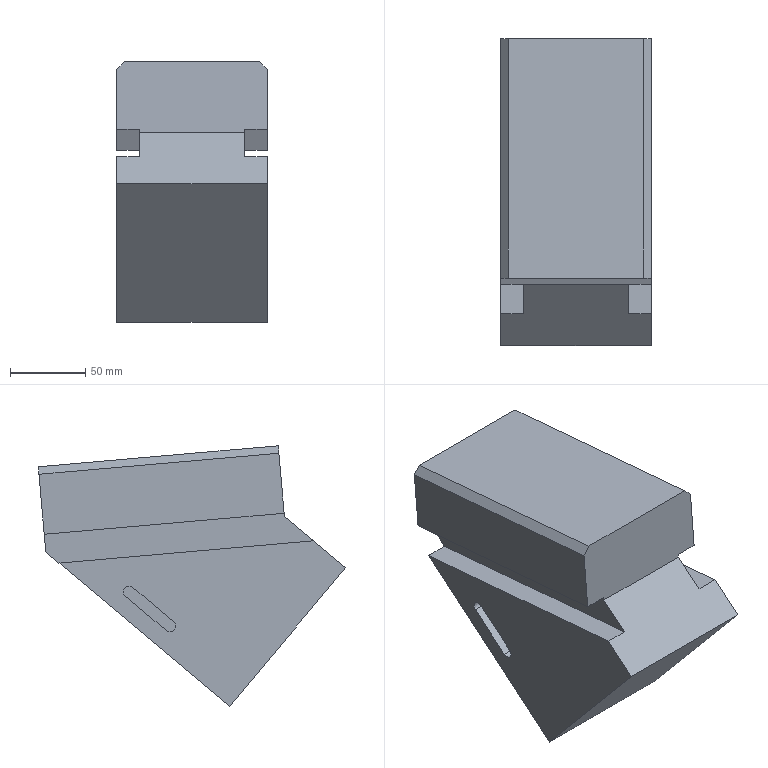Part | NX | features solid 2 | 1 solid | 28 faces | box 100 x 204.22 x 173.003 mm | volume 1996841 mm3 | plane 24 | cylinder 4 | commonest cylinder face diameters 7.661 x4
STEP:
#1=CARTESIAN_POINT('',(-480.,641.399,120.956));
#2=VERTEX_POINT('',#1);
#3=CARTESIAN_POINT('',(-480.,620.,103.));
#4=VERTEX_POINT('',#3);
#5=CARTESIAN_POINT('',(-480.,766.747,226.135));
#6=DIRECTION('',(0.,-0.766,-0.6428));
#7=VECTOR('',#6,1000.);
#8=LINE('',#5,#7);
#9=EDGE_CURVE('',#2,#4,#8,.T.);
#10=ORIENTED_EDGE('',*,*,#9,.T.);
#11=CARTESIAN_POINT('',(-480.,697.135,11.075));
#12=VERTEX_POINT('',#11);
#13=CARTESIAN_POINT('',(-480.,713.253,-8.135));
#14=DIRECTION('',(0.,0.6428,-0.766));
#15=VECTOR('',#14,1000.);
#16=LINE('',#13,#15);
#17=EDGE_CURVE('',#4,#12,#16,.T.);
#18=ORIENTED_EDGE('',*,*,#17,.T.);
#19=CARTESIAN_POINT('',(-480.,810.459,106.165));
#20=VERTEX_POINT('',#19);
#21=CARTESIAN_POINT('',(-480.,843.881,134.21));
#22=DIRECTION('',(0.,-0.766,-0.6428));
#23=VECTOR('',#22,1000.);
#24=LINE('',#21,#23);
#25=EDGE_CURVE('',#20,#12,#24,.T.);
#26=ORIENTED_EDGE('',*,*,#25,.F.);
#27=CARTESIAN_POINT('',(-480.,709.476,115.));
#28=DIRECTION('',(0.,-0.9962,0.08716));
#29=VECTOR('',#28,1000.);
#30=LINE('',#27,#29);
#31=EDGE_CURVE('',#20,#2,#30,.T.);
#32=ORIENTED_EDGE('',*,*,#31,.T.);
#33=EDGE_LOOP('',(#10,#18,#26,#32));
#34=FACE_BOUND('',#33,.T.);
#35=CARTESIAN_POINT('',(-480.,766.324,84.132));
#36=VERTEX_POINT('',#35);
#37=CARTESIAN_POINT('',(-480.,739.242,61.407));
#38=VERTEX_POINT('',#37);
#39=CARTESIAN_POINT('',(-480.,761.4,80.));
#40=DIRECTION('',(0.,-0.766,-0.6428));
#41=VECTOR('',#40,1000.);
#42=LINE('',#39,#41);
#43=EDGE_CURVE('',#36,#38,#42,.T.);
#44=ORIENTED_EDGE('',*,*,#43,.T.);
#45=CARTESIAN_POINT('',(-480.,734.318,67.275));
#46=VERTEX_POINT('',#45);
#47=CARTESIAN_POINT('',(-480.,736.765,64.329));
#48=DIRECTION('',(-1.,0.,0.));
#49=DIRECTION('',(0.,-1.,0.));
#50=AXIS2_PLACEMENT_3D('',#47,#48,#49);
#51=CIRCLE('',#50,3.83);
#52=EDGE_CURVE('',#38,#46,#51,.T.);
#53=ORIENTED_EDGE('',*,*,#52,.T.);
#54=CARTESIAN_POINT('',(-480.,761.4,90.));
#55=VERTEX_POINT('',#54);
#56=CARTESIAN_POINT('',(-480.,761.4,90.));
#57=DIRECTION('',(0.,-0.766,-0.6428));
#58=VECTOR('',#57,1000.);
#59=LINE('',#56,#58);
#60=EDGE_CURVE('',#55,#46,#59,.T.);
#61=ORIENTED_EDGE('',*,*,#60,.F.);
#62=CARTESIAN_POINT('',(-480.,763.874,87.076));
#63=DIRECTION('',(-1.,0.,0.));
#64=DIRECTION('',(0.,-1.,0.));
#65=AXIS2_PLACEMENT_3D('',#62,#63,#64);
#66=CIRCLE('',#65,3.83);
#67=EDGE_CURVE('',#55,#36,#66,.T.);
#68=ORIENTED_EDGE('',*,*,#67,.T.);
#69=EDGE_LOOP('',(#44,#53,#61,#68));
#70=FACE_BOUND('',#69,.T.);
#71=CARTESIAN_POINT('',(-480.,860.,115.));
#72=DIRECTION('',(1.,0.,0.));
#73=DIRECTION('',(0.,0.,-1.));
#74=AXIS2_PLACEMENT_3D('',#71,#72,#73);
#75=PLANE('',#74);
#76=ADVANCED_FACE('',(#34,#70),#75,.T.);
#77=CARTESIAN_POINT('',(-580.,761.4,90.));
#78=VERTEX_POINT('',#77);
#79=CARTESIAN_POINT('',(-580.,766.324,84.132));
#80=VERTEX_POINT('',#79);
#81=CARTESIAN_POINT('',(-580.,763.874,87.076));
#82=DIRECTION('',(-1.,0.,0.));
#83=DIRECTION('',(0.,-1.,0.));
#84=AXIS2_PLACEMENT_3D('',#81,#82,#83);
#85=CIRCLE('',#84,3.83);
#86=EDGE_CURVE('',#78,#80,#85,.T.);
#87=ORIENTED_EDGE('',*,*,#86,.F.);
#88=CARTESIAN_POINT('',(-580.,734.318,67.275));
#89=VERTEX_POINT('',#88);
#90=CARTESIAN_POINT('',(-580.,761.4,90.));
#91=DIRECTION('',(0.,-0.766,-0.6428));
#92=VECTOR('',#91,1000.);
#93=LINE('',#90,#92);
#94=EDGE_CURVE('',#78,#89,#93,.T.);
#95=ORIENTED_EDGE('',*,*,#94,.T.);
#96=CARTESIAN_POINT('',(-580.,739.242,61.407));
#97=VERTEX_POINT('',#96);
#98=CARTESIAN_POINT('',(-580.,736.765,64.329));
#99=DIRECTION('',(-1.,0.,0.));
#100=DIRECTION('',(0.,-1.,0.));
#101=AXIS2_PLACEMENT_3D('',#98,#99,#100);
#102=CIRCLE('',#101,3.83);
#103=EDGE_CURVE('',#97,#89,#102,.T.);
#104=ORIENTED_EDGE('',*,*,#103,.F.);
#105=CARTESIAN_POINT('',(-580.,761.4,80.));
#106=DIRECTION('',(0.,-0.766,-0.6428));
#107=VECTOR('',#106,1000.);
#108=LINE('',#105,#107);
#109=EDGE_CURVE('',#80,#97,#108,.T.);
#110=ORIENTED_EDGE('',*,*,#109,.F.);
#111=EDGE_LOOP('',(#87,#95,#104,#110));
#112=FACE_BOUND('',#111,.T.);
#113=CARTESIAN_POINT('',(-580.,810.459,106.165));
#114=VERTEX_POINT('',#113);
#115=CARTESIAN_POINT('',(-580.,641.399,120.956));
#116=VERTEX_POINT('',#115);
#117=CARTESIAN_POINT('',(-580.,709.476,115.));
#118=DIRECTION('',(0.,-0.9962,0.08716));
#119=VECTOR('',#118,1000.);
#120=LINE('',#117,#119);
#121=EDGE_CURVE('',#114,#116,#120,.T.);
#122=ORIENTED_EDGE('',*,*,#121,.F.);
#123=CARTESIAN_POINT('',(-580.,697.135,11.075));
#124=VERTEX_POINT('',#123);
#125=CARTESIAN_POINT('',(-580.,875.887,161.066));
#126=DIRECTION('',(0.,0.766,0.6428));
#127=VECTOR('',#126,1000.);
#128=LINE('',#125,#127);
#129=EDGE_CURVE('',#124,#114,#128,.T.);
#130=ORIENTED_EDGE('',*,*,#129,.F.);
#131=CARTESIAN_POINT('',(-580.,620.,103.));
#132=VERTEX_POINT('',#131);
#133=CARTESIAN_POINT('',(-580.,681.247,30.009));
#134=DIRECTION('',(0.,-0.6428,0.766));
#135=VECTOR('',#134,1000.);
#136=LINE('',#133,#135);
#137=EDGE_CURVE('',#124,#132,#136,.T.);
#138=ORIENTED_EDGE('',*,*,#137,.T.);
#139=CARTESIAN_POINT('',(-580.,798.753,252.991));
#140=DIRECTION('',(0.,0.766,0.6428));
#141=VECTOR('',#140,1000.);
#142=LINE('',#139,#141);
#143=EDGE_CURVE('',#132,#116,#142,.T.);
#144=ORIENTED_EDGE('',*,*,#143,.T.);
#145=EDGE_LOOP('',(#122,#130,#138,#144));
#146=FACE_BOUND('',#145,.T.);
#147=CARTESIAN_POINT('',(-580.,860.,180.));
#148=DIRECTION('',(-1.,0.,0.));
#149=DIRECTION('',(0.,1.,0.));
#150=AXIS2_PLACEMENT_3D('',#147,#148,#149);
#151=PLANE('',#150);
#152=ADVANCED_FACE('',(#112,#146),#151,.T.);
#153=CARTESIAN_POINT('',(-480.,823.784,165.152));
#154=VERTEX_POINT('',#153);
#155=CARTESIAN_POINT('',(-480.,820.298,125.304));
#156=VERTEX_POINT('',#155);
#157=CARTESIAN_POINT('',(-480.,819.705,118.525));
#158=DIRECTION('',(0.,-0.08716,-0.9962));
#159=VECTOR('',#158,1000.);
#160=LINE('',#157,#159);
#161=EDGE_CURVE('',#154,#156,#160,.T.);
#162=ORIENTED_EDGE('',*,*,#161,.F.);
#163=CARTESIAN_POINT('',(-480.,664.393,179.097));
#164=VERTEX_POINT('',#163);
#165=CARTESIAN_POINT('',(-480.,864.079,161.627));
#166=DIRECTION('',(0.,0.9962,-0.08716));
#167=VECTOR('',#166,1000.);
#168=LINE('',#165,#167);
#169=EDGE_CURVE('',#164,#154,#168,.T.);
#170=ORIENTED_EDGE('',*,*,#169,.F.);
#171=CARTESIAN_POINT('',(-480.,660.907,139.249));
#172=VERTEX_POINT('',#171);
#173=CARTESIAN_POINT('',(-480.,660.314,132.47));
#174=DIRECTION('',(0.,-0.08716,-0.9962));
#175=VECTOR('',#174,1000.);
#176=LINE('',#173,#175);
#177=EDGE_CURVE('',#164,#172,#176,.T.);
#178=ORIENTED_EDGE('',*,*,#177,.T.);
#179=CARTESIAN_POINT('',(-480.,820.,125.33));
#180=DIRECTION('',(0.,0.9962,-0.08716));
#181=VECTOR('',#180,1000.);
#182=LINE('',#179,#181);
#183=EDGE_CURVE('',#172,#156,#182,.T.);
#184=ORIENTED_EDGE('',*,*,#183,.T.);
#185=EDGE_LOOP('',(#162,#170,#178,#184));
#186=FACE_BOUND('',#185,.T.);
#187=CARTESIAN_POINT('',(-480.,860.,115.));
#188=DIRECTION('',(1.,0.,0.));
#189=DIRECTION('',(0.,0.,-1.));
#190=AXIS2_PLACEMENT_3D('',#187,#188,#189);
#191=PLANE('',#190);
#192=ADVANCED_FACE('',(#186),#191,.T.);
#193=CARTESIAN_POINT('',(-580.,820.298,125.304));
#194=VERTEX_POINT('',#193);
#195=CARTESIAN_POINT('',(-565.,820.298,125.304));
#196=VERTEX_POINT('',#195);
#197=CARTESIAN_POINT('',(-580.,820.298,125.304));
#198=DIRECTION('',(1.,0.,0.));
#199=VECTOR('',#198,1000.);
#200=LINE('',#197,#199);
#201=EDGE_CURVE('',#194,#196,#200,.T.);
#202=ORIENTED_EDGE('',*,*,#201,.F.);
#203=CARTESIAN_POINT('',(-580.,823.784,165.152));
#204=VERTEX_POINT('',#203);
#205=CARTESIAN_POINT('',(-580.,825.348,183.032));
#206=DIRECTION('',(0.,0.08716,0.9962));
#207=VECTOR('',#206,1000.);
#208=LINE('',#205,#207);
#209=EDGE_CURVE('',#194,#204,#208,.T.);
#210=ORIENTED_EDGE('',*,*,#209,.T.);
#211=CARTESIAN_POINT('',(-575.,824.22,170.133));
#212=VERTEX_POINT('',#211);
#213=CARTESIAN_POINT('',(-652.5,817.465,92.928));
#214=DIRECTION('',(0.7071,0.06163,0.7044));
#215=VECTOR('',#214,1000.);
#216=LINE('',#213,#215);
#217=EDGE_CURVE('',#212,#204,#216,.F.);
#218=ORIENTED_EDGE('',*,*,#217,.F.);
#219=CARTESIAN_POINT('',(-485.,824.22,170.133));
#220=VERTEX_POINT('',#219);
#221=CARTESIAN_POINT('',(-730.,824.22,170.133));
#222=DIRECTION('',(1.,0.,0.));
#223=VECTOR('',#222,1000.);
#224=LINE('',#221,#223);
#225=EDGE_CURVE('',#212,#220,#224,.T.);
#226=ORIENTED_EDGE('',*,*,#225,.T.);
#227=CARTESIAN_POINT('',(-607.5,834.896,292.167));
#228=DIRECTION('',(0.7071,-0.06163,-0.7044));
#229=VECTOR('',#228,1000.);
#230=LINE('',#227,#229);
#231=EDGE_CURVE('',#154,#220,#230,.F.);
#232=ORIENTED_EDGE('',*,*,#231,.F.);
#233=ORIENTED_EDGE('',*,*,#161,.T.);
#234=CARTESIAN_POINT('',(-495.,820.298,125.304));
#235=VERTEX_POINT('',#234);
#236=CARTESIAN_POINT('',(-480.,820.298,125.304));
#237=DIRECTION('',(-1.,0.,0.));
#238=VECTOR('',#237,1000.);
#239=LINE('',#236,#238);
#240=EDGE_CURVE('',#156,#235,#239,.T.);
#241=ORIENTED_EDGE('',*,*,#240,.T.);
#242=CARTESIAN_POINT('',(-495.,819.27,113.559));
#243=VERTEX_POINT('',#242);
#244=CARTESIAN_POINT('',(-495.,824.22,170.133));
#245=DIRECTION('',(0.,-0.08716,-0.9962));
#246=VECTOR('',#245,1000.);
#247=LINE('',#244,#246);
#248=EDGE_CURVE('',#235,#243,#247,.T.);
#249=ORIENTED_EDGE('',*,*,#248,.T.);
#250=CARTESIAN_POINT('',(-565.,819.27,113.559));
#251=VERTEX_POINT('',#250);
#252=CARTESIAN_POINT('',(-730.,819.27,113.559));
#253=DIRECTION('',(1.,0.,0.));
#254=VECTOR('',#253,1000.);
#255=LINE('',#252,#254);
#256=EDGE_CURVE('',#251,#243,#255,.T.);
#257=ORIENTED_EDGE('',*,*,#256,.F.);
#258=CARTESIAN_POINT('',(-565.,824.22,170.133));
#259=DIRECTION('',(0.,-0.08716,-0.9962));
#260=VECTOR('',#259,1000.);
#261=LINE('',#258,#260);
#262=EDGE_CURVE('',#196,#251,#261,.T.);
#263=ORIENTED_EDGE('',*,*,#262,.F.);
#264=EDGE_LOOP('',(#202,#210,#218,#226,#232,#233,#241,#249,#257,#263));
#265=FACE_BOUND('',#264,.T.);
#266=CARTESIAN_POINT('',(-730.,824.22,170.133));
#267=DIRECTION('',(0.,0.9962,-0.08716));
#268=DIRECTION('',(0.,-0.08716,-0.9962));
#269=AXIS2_PLACEMENT_3D('',#266,#267,#268);
#270=PLANE('',#269);
#271=ADVANCED_FACE('',(#265),#270,.T.);
#272=CARTESIAN_POINT('',(-565.,660.907,139.249));
#273=VERTEX_POINT('',#272);
#274=CARTESIAN_POINT('',(-565.,660.725,137.172));
#275=VERTEX_POINT('',#274);
#276=CARTESIAN_POINT('',(-565.,660.907,139.249));
#277=DIRECTION('',(0.,-0.08716,-0.9962));
#278=VECTOR('',#277,1000.);
#279=LINE('',#276,#278);
#280=EDGE_CURVE('',#273,#275,#279,.T.);
#281=ORIENTED_EDGE('',*,*,#280,.T.);
#282=CARTESIAN_POINT('',(-495.,660.725,137.172));
#283=VERTEX_POINT('',#282);
#284=CARTESIAN_POINT('',(-730.,660.725,137.172));
#285=DIRECTION('',(1.,0.,0.));
#286=VECTOR('',#285,1000.);
#287=LINE('',#284,#286);
#288=EDGE_CURVE('',#275,#283,#287,.T.);
#289=ORIENTED_EDGE('',*,*,#288,.T.);
#290=CARTESIAN_POINT('',(-495.,660.907,139.249));
#291=VERTEX_POINT('',#290);
#292=CARTESIAN_POINT('',(-495.,660.907,139.249));
#293=DIRECTION('',(0.,-0.08716,-0.9962));
#294=VECTOR('',#293,1000.);
#295=LINE('',#292,#294);
#296=EDGE_CURVE('',#291,#283,#295,.T.);
#297=ORIENTED_EDGE('',*,*,#296,.F.);
#298=CARTESIAN_POINT('',(-480.,660.907,139.249));
#299=DIRECTION('',(-1.,0.,0.));
#300=VECTOR('',#299,1000.);
#301=LINE('',#298,#300);
#302=EDGE_CURVE('',#172,#291,#301,.T.);
#303=ORIENTED_EDGE('',*,*,#302,.F.);
#304=ORIENTED_EDGE('',*,*,#177,.F.);
#305=CARTESIAN_POINT('',(-485.,664.829,184.078));
#306=VERTEX_POINT('',#305);
#307=CARTESIAN_POINT('',(-480.,664.393,179.097));
#308=DIRECTION('',(-0.7071,0.06163,0.7044));
#309=VECTOR('',#308,1000.);
#310=LINE('',#307,#309);
#311=EDGE_CURVE('',#306,#164,#310,.F.);
#312=ORIENTED_EDGE('',*,*,#311,.F.);
#313=CARTESIAN_POINT('',(-575.,664.829,184.078));
#314=VERTEX_POINT('',#313);
#315=CARTESIAN_POINT('',(-730.,664.829,184.078));
#316=DIRECTION('',(1.,0.,0.));
#317=VECTOR('',#316,1000.);
#318=LINE('',#315,#317);
#319=EDGE_CURVE('',#314,#306,#318,.T.);
#320=ORIENTED_EDGE('',*,*,#319,.F.);
#321=CARTESIAN_POINT('',(-580.,664.393,179.097));
#322=VERTEX_POINT('',#321);
#323=CARTESIAN_POINT('',(-580.,664.393,179.097));
#324=DIRECTION('',(-0.7071,-0.06163,-0.7044));
#325=VECTOR('',#324,1000.);
#326=LINE('',#323,#325);
#327=EDGE_CURVE('',#322,#314,#326,.F.);
#328=ORIENTED_EDGE('',*,*,#327,.F.);
#329=CARTESIAN_POINT('',(-580.,660.907,139.249));
#330=VERTEX_POINT('',#329);
#331=CARTESIAN_POINT('',(-580.,665.957,196.977));
#332=DIRECTION('',(0.,0.08716,0.9962));
#333=VECTOR('',#332,1000.);
#334=LINE('',#331,#333);
#335=EDGE_CURVE('',#330,#322,#334,.T.);
#336=ORIENTED_EDGE('',*,*,#335,.F.);
#337=CARTESIAN_POINT('',(-580.,660.907,139.249));
#338=DIRECTION('',(1.,0.,0.));
#339=VECTOR('',#338,1000.);
#340=LINE('',#337,#339);
#341=EDGE_CURVE('',#330,#273,#340,.T.);
#342=ORIENTED_EDGE('',*,*,#341,.T.);
#343=EDGE_LOOP('',(#281,#289,#297,#303,#304,#312,#320,#328,#336,#342));
#344=FACE_BOUND('',#343,.T.);
#345=CARTESIAN_POINT('',(-730.,660.907,139.249));
#346=DIRECTION('',(0.,0.9962,-0.08716));
#347=DIRECTION('',(0.,-0.08716,-0.9962));
#348=AXIS2_PLACEMENT_3D('',#345,#346,#347);
#349=PLANE('',#348);
#350=ADVANCED_FACE('',(#344),#349,.F.);
#351=ORIENTED_EDGE('',*,*,#143,.F.);
#352=CARTESIAN_POINT('',(-730.,620.,103.));
#353=DIRECTION('',(1.,0.,0.));
#354=VECTOR('',#353,1000.);
#355=LINE('',#352,#354);
#356=EDGE_CURVE('',#132,#4,#355,.T.);
#357=ORIENTED_EDGE('',*,*,#356,.T.);
#358=ORIENTED_EDGE('',*,*,#9,.F.);
#359=CARTESIAN_POINT('',(-495.,641.399,120.956));
#360=VERTEX_POINT('',#359);
#361=CARTESIAN_POINT('',(-730.,641.399,120.956));
#362=DIRECTION('',(-1.,0.,0.));
#363=VECTOR('',#362,1000.);
#364=LINE('',#361,#363);
#365=EDGE_CURVE('',#2,#360,#364,.T.);
#366=ORIENTED_EDGE('',*,*,#365,.T.);
#367=CARTESIAN_POINT('',(-495.,660.725,137.172));
#368=DIRECTION('',(0.,-0.766,-0.6428));
#369=VECTOR('',#368,1000.);
#370=LINE('',#367,#369);
#371=EDGE_CURVE('',#283,#360,#370,.T.);
#372=ORIENTED_EDGE('',*,*,#371,.F.);
#373=ORIENTED_EDGE('',*,*,#288,.F.);
#374=CARTESIAN_POINT('',(-565.,641.399,120.956));
#375=VERTEX_POINT('',#374);
#376=CARTESIAN_POINT('',(-565.,660.725,137.172));
#377=DIRECTION('',(0.,-0.766,-0.6428));
#378=VECTOR('',#377,1000.);
#379=LINE('',#376,#378);
#380=EDGE_CURVE('',#275,#375,#379,.T.);
#381=ORIENTED_EDGE('',*,*,#380,.T.);
#382=CARTESIAN_POINT('',(-730.,641.399,120.956));
#383=DIRECTION('',(1.,0.,0.));
#384=VECTOR('',#383,1000.);
#385=LINE('',#382,#384);
#386=EDGE_CURVE('',#116,#375,#385,.T.);
#387=ORIENTED_EDGE('',*,*,#386,.F.);
#388=EDGE_LOOP('',(#351,#357,#358,#366,#372,#373,#381,#387));
#389=FACE_BOUND('',#388,.T.);
#390=CARTESIAN_POINT('',(-730.,660.725,137.172));
#391=DIRECTION('',(0.,0.6428,-0.766));
#392=DIRECTION('',(0.,-0.766,-0.6428));
#393=AXIS2_PLACEMENT_3D('',#390,#391,#392);
#394=PLANE('',#393);
#395=ADVANCED_FACE('',(#389),#394,.F.);
#396=CARTESIAN_POINT('',(-565.,810.459,106.165));
#397=VERTEX_POINT('',#396);
#398=CARTESIAN_POINT('',(-580.,810.459,106.165));
#399=DIRECTION('',(1.,0.,0.));
#400=VECTOR('',#399,1000.);
#401=LINE('',#398,#400);
#402=EDGE_CURVE('',#114,#397,#401,.T.);
#403=ORIENTED_EDGE('',*,*,#402,.T.);
#404=CARTESIAN_POINT('',(-565.,819.27,113.559));
#405=DIRECTION('',(0.,-0.766,-0.6428));
#406=VECTOR('',#405,1000.);
#407=LINE('',#404,#406);
#408=EDGE_CURVE('',#251,#397,#407,.T.);
#409=ORIENTED_EDGE('',*,*,#408,.F.);
#410=ORIENTED_EDGE('',*,*,#256,.T.);
#411=CARTESIAN_POINT('',(-495.,810.459,106.165));
#412=VERTEX_POINT('',#411);
#413=CARTESIAN_POINT('',(-495.,819.27,113.559));
#414=DIRECTION('',(0.,-0.766,-0.6428));
#415=VECTOR('',#414,1000.);
#416=LINE('',#413,#415);
#417=EDGE_CURVE('',#243,#412,#416,.T.);
#418=ORIENTED_EDGE('',*,*,#417,.T.);
#419=CARTESIAN_POINT('',(-480.,810.459,106.165));
#420=DIRECTION('',(-1.,0.,0.));
#421=VECTOR('',#420,1000.);
#422=LINE('',#419,#421);
#423=EDGE_CURVE('',#20,#412,#422,.T.);
#424=ORIENTED_EDGE('',*,*,#423,.F.);
#425=ORIENTED_EDGE('',*,*,#25,.T.);
#426=CARTESIAN_POINT('',(-730.,697.135,11.075));
#427=DIRECTION('',(1.,0.,0.));
#428=VECTOR('',#427,1000.);
#429=LINE('',#426,#428);
#430=EDGE_CURVE('',#124,#12,#429,.T.);
#431=ORIENTED_EDGE('',*,*,#430,.F.);
#432=ORIENTED_EDGE('',*,*,#129,.T.);
#433=EDGE_LOOP('',(#403,#409,#410,#418,#424,#425,#431,#432));
#434=FACE_BOUND('',#433,.T.);
#435=CARTESIAN_POINT('',(-730.,819.27,113.559));
#436=DIRECTION('',(0.,0.6428,-0.766));
#437=DIRECTION('',(0.,-0.766,-0.6428));
#438=AXIS2_PLACEMENT_3D('',#435,#436,#437);
#439=PLANE('',#438);
#440=ADVANCED_FACE('',(#434),#439,.T.);
#441=ORIENTED_EDGE('',*,*,#319,.T.);
#442=CARTESIAN_POINT('',(-485.,654.867,184.95));
#443=DIRECTION('',(0.,-0.9962,0.08716));
#444=VECTOR('',#443,1000.);
#445=LINE('',#442,#444);
#446=EDGE_CURVE('',#220,#306,#445,.T.);
#447=ORIENTED_EDGE('',*,*,#446,.F.);
#448=ORIENTED_EDGE('',*,*,#225,.F.);
#449=CARTESIAN_POINT('',(-575.,654.867,184.95));
#450=DIRECTION('',(0.,0.9962,-0.08716));
#451=VECTOR('',#450,1000.);
#452=LINE('',#449,#451);
#453=EDGE_CURVE('',#314,#212,#452,.T.);
#454=ORIENTED_EDGE('',*,*,#453,.F.);
#455=EDGE_LOOP('',(#441,#447,#448,#454));
#456=FACE_BOUND('',#455,.T.);
#457=CARTESIAN_POINT('',(-730.,654.867,184.95));
#458=DIRECTION('',(0.,0.08716,0.9962));
#459=DIRECTION('',(0.,0.9962,-0.08716));
#460=AXIS2_PLACEMENT_3D('',#457,#458,#459);
#461=PLANE('',#460);
#462=ADVANCED_FACE('',(#456),#461,.T.);
#463=ORIENTED_EDGE('',*,*,#430,.T.);
#464=ORIENTED_EDGE('',*,*,#17,.F.);
#465=ORIENTED_EDGE('',*,*,#356,.F.);
#466=ORIENTED_EDGE('',*,*,#137,.F.);
#467=EDGE_LOOP('',(#463,#464,#465,#466));
#468=FACE_BOUND('',#467,.T.);
#469=CARTESIAN_POINT('',(-730.,620.,103.));
#470=DIRECTION('',(0.,0.766,0.6428));
#471=DIRECTION('',(0.,0.6428,-0.766));
#472=AXIS2_PLACEMENT_3D('',#469,#470,#471);
#473=PLANE('',#472);
#474=ADVANCED_FACE('',(#468),#473,.F.);
#475=CARTESIAN_POINT('',(-580.,820.,125.33));
#476=DIRECTION('',(0.,0.9962,-0.08716));
#477=VECTOR('',#476,1000.);
#478=LINE('',#475,#477);
#479=EDGE_CURVE('',#330,#194,#478,.T.);
#480=ORIENTED_EDGE('',*,*,#479,.F.);
#481=ORIENTED_EDGE('',*,*,#335,.T.);
#482=CARTESIAN_POINT('',(-580.,858.436,162.12));
#483=DIRECTION('',(0.,-0.9962,0.08716));
#484=VECTOR('',#483,1000.);
#485=LINE('',#482,#484);
#486=EDGE_CURVE('',#204,#322,#485,.T.);
#487=ORIENTED_EDGE('',*,*,#486,.F.);
#488=ORIENTED_EDGE('',*,*,#209,.F.);
#489=EDGE_LOOP('',(#480,#481,#487,#488));
#490=FACE_BOUND('',#489,.T.);
#491=CARTESIAN_POINT('',(-580.,860.,180.));
#492=DIRECTION('',(-1.,0.,0.));
#493=DIRECTION('',(0.,1.,0.));
#494=AXIS2_PLACEMENT_3D('',#491,#492,#493);
#495=PLANE('',#494);
#496=ADVANCED_FACE('',(#490),#495,.T.);
#497=ORIENTED_EDGE('',*,*,#217,.T.);
#498=ORIENTED_EDGE('',*,*,#486,.T.);
#499=ORIENTED_EDGE('',*,*,#327,.T.);
#500=ORIENTED_EDGE('',*,*,#453,.T.);
#501=EDGE_LOOP('',(#497,#498,#499,#500));
#502=FACE_BOUND('',#501,.T.);
#503=CARTESIAN_POINT('',(-580.,858.436,162.12));
#504=DIRECTION('',(0.7071,-0.06163,-0.7044));
#505=DIRECTION('',(-0.7058,0.,-0.7085));
#506=AXIS2_PLACEMENT_3D('',#503,#504,#505);
#507=PLANE('',#506);
#508=ADVANCED_FACE('',(#502),#507,.F.);
#509=ORIENTED_EDGE('',*,*,#311,.T.);
#510=ORIENTED_EDGE('',*,*,#169,.T.);
#511=ORIENTED_EDGE('',*,*,#231,.T.);
#512=ORIENTED_EDGE('',*,*,#446,.T.);
#513=EDGE_LOOP('',(#509,#510,#511,#512));
#514=FACE_BOUND('',#513,.T.);
#515=CARTESIAN_POINT('',(-480.,864.079,161.627));
#516=DIRECTION('',(-0.7071,-0.06163,-0.7044));
#517=DIRECTION('',(-0.7058,0.,0.7085));
#518=AXIS2_PLACEMENT_3D('',#515,#516,#517);
#519=PLANE('',#518);
#520=ADVANCED_FACE('',(#514),#519,.F.);
#521=CARTESIAN_POINT('',(-495.,709.476,115.));
#522=DIRECTION('',(0.,-0.9962,0.08716));
#523=VECTOR('',#522,1000.);
#524=LINE('',#521,#523);
#525=EDGE_CURVE('',#412,#360,#524,.T.);
#526=ORIENTED_EDGE('',*,*,#525,.T.);
#527=ORIENTED_EDGE('',*,*,#365,.F.);
#528=ORIENTED_EDGE('',*,*,#31,.F.);
#529=ORIENTED_EDGE('',*,*,#423,.T.);
#530=EDGE_LOOP('',(#526,#527,#528,#529));
#531=FACE_BOUND('',#530,.T.);
#532=CARTESIAN_POINT('',(-480.,709.476,115.));
#533=DIRECTION('',(0.,0.08716,0.9962));
#534=DIRECTION('',(0.,0.9962,-0.08716));
#535=AXIS2_PLACEMENT_3D('',#532,#533,#534);
#536=PLANE('',#535);
#537=ADVANCED_FACE('',(#531),#536,.T.);
#538=CARTESIAN_POINT('',(-495.,820.,125.33));
#539=DIRECTION('',(0.,0.9962,-0.08716));
#540=VECTOR('',#539,1000.);
#541=LINE('',#538,#540);
#542=EDGE_CURVE('',#291,#235,#541,.T.);
#543=ORIENTED_EDGE('',*,*,#542,.T.);
#544=ORIENTED_EDGE('',*,*,#240,.F.);
#545=ORIENTED_EDGE('',*,*,#183,.F.);
#546=ORIENTED_EDGE('',*,*,#302,.T.);
#547=EDGE_LOOP('',(#543,#544,#545,#546));
#548=FACE_BOUND('',#547,.T.);
#549=CARTESIAN_POINT('',(-480.,820.,125.33));
#550=DIRECTION('',(0.,-0.08716,-0.9962));
#551=DIRECTION('',(0.,-0.9962,0.08716));
#552=AXIS2_PLACEMENT_3D('',#549,#550,#551);
#553=PLANE('',#552);
#554=ADVANCED_FACE('',(#548),#553,.T.);
#555=ORIENTED_EDGE('',*,*,#525,.F.);
#556=ORIENTED_EDGE('',*,*,#417,.F.);
#557=ORIENTED_EDGE('',*,*,#248,.F.);
#558=ORIENTED_EDGE('',*,*,#542,.F.);
#559=ORIENTED_EDGE('',*,*,#296,.T.);
#560=ORIENTED_EDGE('',*,*,#371,.T.);
#561=EDGE_LOOP('',(#555,#556,#557,#558,#559,#560));
#562=FACE_BOUND('',#561,.T.);
#563=CARTESIAN_POINT('',(-495.,734.642,118.578));
#564=DIRECTION('',(-1.,0.,0.));
#565=DIRECTION('',(0.,1.,0.));
#566=AXIS2_PLACEMENT_3D('',#563,#564,#565);
#567=PLANE('',#566);
#568=ADVANCED_FACE('',(#562),#567,.F.);
#569=CARTESIAN_POINT('',(-565.,709.476,115.));
#570=DIRECTION('',(0.,-0.9962,0.08716));
#571=VECTOR('',#570,1000.);
#572=LINE('',#569,#571);
#573=EDGE_CURVE('',#397,#375,#572,.T.);
#574=ORIENTED_EDGE('',*,*,#573,.F.);
#575=ORIENTED_EDGE('',*,*,#402,.F.);
#576=ORIENTED_EDGE('',*,*,#121,.T.);
#577=ORIENTED_EDGE('',*,*,#386,.T.);
#578=EDGE_LOOP('',(#574,#575,#576,#577));
#579=FACE_BOUND('',#578,.T.);
#580=CARTESIAN_POINT('',(-580.,709.476,115.));
#581=DIRECTION('',(0.,-0.08716,-0.9962));
#582=DIRECTION('',(0.,-0.9962,0.08716));
#583=AXIS2_PLACEMENT_3D('',#580,#581,#582);
#584=PLANE('',#583);
#585=ADVANCED_FACE('',(#579),#584,.F.);
#586=CARTESIAN_POINT('',(-565.,820.,125.33));
#587=DIRECTION('',(0.,0.9962,-0.08716));
#588=VECTOR('',#587,1000.);
#589=LINE('',#586,#588);
#590=EDGE_CURVE('',#273,#196,#589,.T.);
#591=ORIENTED_EDGE('',*,*,#590,.F.);
#592=ORIENTED_EDGE('',*,*,#341,.F.);
#593=ORIENTED_EDGE('',*,*,#479,.T.);
#594=ORIENTED_EDGE('',*,*,#201,.T.);
#595=EDGE_LOOP('',(#591,#592,#593,#594));
#596=FACE_BOUND('',#595,.T.);
#597=CARTESIAN_POINT('',(-580.,820.,125.33));
#598=DIRECTION('',(0.,0.08716,0.9962));
#599=DIRECTION('',(0.,0.9962,-0.08716));
#600=AXIS2_PLACEMENT_3D('',#597,#598,#599);
#601=PLANE('',#600);
#602=ADVANCED_FACE('',(#596),#601,.F.);
#603=ORIENTED_EDGE('',*,*,#573,.T.);
#604=ORIENTED_EDGE('',*,*,#380,.F.);
#605=ORIENTED_EDGE('',*,*,#280,.F.);
#606=ORIENTED_EDGE('',*,*,#590,.T.);
#607=ORIENTED_EDGE('',*,*,#262,.T.);
#608=ORIENTED_EDGE('',*,*,#408,.T.);
#609=EDGE_LOOP('',(#603,#604,#605,#606,#607,#608));
#610=FACE_BOUND('',#609,.T.);
#611=CARTESIAN_POINT('',(-565.,734.642,118.578));
#612=DIRECTION('',(-1.,0.,0.));
#613=DIRECTION('',(0.,1.,0.));
#614=AXIS2_PLACEMENT_3D('',#611,#612,#613);
#615=PLANE('',#614);
#616=ADVANCED_FACE('',(#610),#615,.T.);
#617=CARTESIAN_POINT('',(-570.,761.4,90.));
#618=VERTEX_POINT('',#617);
#619=CARTESIAN_POINT('',(-570.,766.324,84.132));
#620=VERTEX_POINT('',#619);
#621=CARTESIAN_POINT('',(-570.,763.874,87.076));
#622=DIRECTION('',(-1.,0.,0.));
#623=DIRECTION('',(0.,-1.,0.));
#624=AXIS2_PLACEMENT_3D('',#621,#622,#623);
#625=CIRCLE('',#624,3.83);
#626=EDGE_CURVE('',#618,#620,#625,.T.);
#627=ORIENTED_EDGE('',*,*,#626,.F.);
#628=CARTESIAN_POINT('',(-580.,761.4,90.));
#629=DIRECTION('',(1.,0.,0.));
#630=VECTOR('',#629,1000.);
#631=LINE('',#628,#630);
#632=EDGE_CURVE('',#78,#618,#631,.T.);
#633=ORIENTED_EDGE('',*,*,#632,.F.);
#634=ORIENTED_EDGE('',*,*,#86,.T.);
#635=CARTESIAN_POINT('',(-580.,766.324,84.132));
#636=DIRECTION('',(1.,0.,0.));
#637=VECTOR('',#636,1000.);
#638=LINE('',#635,#637);
#639=EDGE_CURVE('',#80,#620,#638,.T.);
#640=ORIENTED_EDGE('',*,*,#639,.T.);
#641=EDGE_LOOP('',(#627,#633,#634,#640));
#642=FACE_BOUND('',#641,.T.);
#643=CARTESIAN_POINT('',(-580.,763.874,87.076));
#644=DIRECTION('',(1.,0.,0.));
#645=DIRECTION('',(0.,-1.,0.));
#646=AXIS2_PLACEMENT_3D('',#643,#644,#645);
#647=CYLINDRICAL_SURFACE('',#646,3.83);
#648=ADVANCED_FACE('',(#642),#647,.F.);
#649=CARTESIAN_POINT('',(-570.,739.242,61.407));
#650=VERTEX_POINT('',#649);
#651=CARTESIAN_POINT('',(-570.,761.4,80.));
#652=DIRECTION('',(0.,-0.766,-0.6428));
#653=VECTOR('',#652,1000.);
#654=LINE('',#651,#653);
#655=EDGE_CURVE('',#620,#650,#654,.T.);
#656=ORIENTED_EDGE('',*,*,#655,.F.);
#657=ORIENTED_EDGE('',*,*,#639,.F.);
#658=ORIENTED_EDGE('',*,*,#109,.T.);
#659=CARTESIAN_POINT('',(-580.,739.242,61.407));
#660=DIRECTION('',(1.,0.,0.));
#661=VECTOR('',#660,1000.);
#662=LINE('',#659,#661);
#663=EDGE_CURVE('',#97,#650,#662,.T.);
#664=ORIENTED_EDGE('',*,*,#663,.T.);
#665=EDGE_LOOP('',(#656,#657,#658,#664));
#666=FACE_BOUND('',#665,.T.);
#667=CARTESIAN_POINT('',(-580.,761.4,80.));
#668=DIRECTION('',(0.,0.6428,-0.766));
#669=DIRECTION('',(0.,-0.766,-0.6428));
#670=AXIS2_PLACEMENT_3D('',#667,#668,#669);
#671=PLANE('',#670);
#672=ADVANCED_FACE('',(#666),#671,.F.);
#673=CARTESIAN_POINT('',(-570.,734.318,67.275));
#674=VERTEX_POINT('',#673);
#675=CARTESIAN_POINT('',(-570.,736.765,64.329));
#676=DIRECTION('',(-1.,0.,0.));
#677=DIRECTION('',(0.,-1.,0.));
#678=AXIS2_PLACEMENT_3D('',#675,#676,#677);
#679=CIRCLE('',#678,3.83);
#680=EDGE_CURVE('',#650,#674,#679,.T.);
#681=ORIENTED_EDGE('',*,*,#680,.F.);
#682=ORIENTED_EDGE('',*,*,#663,.F.);
#683=ORIENTED_EDGE('',*,*,#103,.T.);
#684=CARTESIAN_POINT('',(-580.,734.318,67.275));
#685=DIRECTION('',(1.,0.,0.));
#686=VECTOR('',#685,1000.);
#687=LINE('',#684,#686);
#688=EDGE_CURVE('',#89,#674,#687,.T.);
#689=ORIENTED_EDGE('',*,*,#688,.T.);
#690=EDGE_LOOP('',(#681,#682,#683,#689));
#691=FACE_BOUND('',#690,.T.);
#692=CARTESIAN_POINT('',(-580.,736.765,64.329));
#693=DIRECTION('',(1.,0.,0.));
#694=DIRECTION('',(0.,-1.,0.));
#695=AXIS2_PLACEMENT_3D('',#692,#693,#694);
#696=CYLINDRICAL_SURFACE('',#695,3.83);
#697=ADVANCED_FACE('',(#691),#696,.F.);
#698=CARTESIAN_POINT('',(-570.,761.4,90.));
#699=DIRECTION('',(0.,-0.766,-0.6428));
#700=VECTOR('',#699,1000.);
#701=LINE('',#698,#700);
#702=EDGE_CURVE('',#618,#674,#701,.T.);
#703=ORIENTED_EDGE('',*,*,#702,.T.);
#704=ORIENTED_EDGE('',*,*,#688,.F.);
#705=ORIENTED_EDGE('',*,*,#94,.F.);
#706=ORIENTED_EDGE('',*,*,#632,.T.);
#707=EDGE_LOOP('',(#703,#704,#705,#706));
#708=FACE_BOUND('',#707,.T.);
#709=CARTESIAN_POINT('',(-580.,761.4,90.));
#710=DIRECTION('',(0.,0.6428,-0.766));
#711=DIRECTION('',(0.,-0.766,-0.6428));
#712=AXIS2_PLACEMENT_3D('',#709,#710,#711);
#713=PLANE('',#712);
#714=ADVANCED_FACE('',(#708),#713,.T.);
#715=ORIENTED_EDGE('',*,*,#626,.T.);
#716=ORIENTED_EDGE('',*,*,#655,.T.);
#717=ORIENTED_EDGE('',*,*,#680,.T.);
#718=ORIENTED_EDGE('',*,*,#702,.F.);
#719=EDGE_LOOP('',(#715,#716,#717,#718));
#720=FACE_BOUND('',#719,.T.);
#721=CARTESIAN_POINT('',(-570.,763.874,87.076));
#722=DIRECTION('',(1.,0.,0.));
#723=DIRECTION('',(0.,-1.,0.));
#724=AXIS2_PLACEMENT_3D('',#721,#722,#723);
#725=PLANE('',#724);
#726=ADVANCED_FACE('',(#720),#725,.F.);
#727=CARTESIAN_POINT('',(-490.,761.4,90.));
#728=VERTEX_POINT('',#727);
#729=CARTESIAN_POINT('',(-490.,766.324,84.132));
#730=VERTEX_POINT('',#729);
#731=CARTESIAN_POINT('',(-490.,763.874,87.076));
#732=DIRECTION('',(-1.,0.,0.));
#733=DIRECTION('',(0.,-1.,0.));
#734=AXIS2_PLACEMENT_3D('',#731,#732,#733);
#735=CIRCLE('',#734,3.83);
#736=EDGE_CURVE('',#728,#730,#735,.T.);
#737=ORIENTED_EDGE('',*,*,#736,.T.);
#738=CARTESIAN_POINT('',(-480.,766.324,84.132));
#739=DIRECTION('',(-1.,0.,0.));
#740=VECTOR('',#739,1000.);
#741=LINE('',#738,#740);
#742=EDGE_CURVE('',#36,#730,#741,.T.);
#743=ORIENTED_EDGE('',*,*,#742,.F.);
#744=ORIENTED_EDGE('',*,*,#67,.F.);
#745=CARTESIAN_POINT('',(-480.,761.4,90.));
#746=DIRECTION('',(-1.,0.,0.));
#747=VECTOR('',#746,1000.);
#748=LINE('',#745,#747);
#749=EDGE_CURVE('',#55,#728,#748,.T.);
#750=ORIENTED_EDGE('',*,*,#749,.T.);
#751=EDGE_LOOP('',(#737,#743,#744,#750));
#752=FACE_BOUND('',#751,.T.);
#753=CARTESIAN_POINT('',(-480.,763.874,87.076));
#754=DIRECTION('',(-1.,0.,0.));
#755=DIRECTION('',(0.,1.,0.));
#756=AXIS2_PLACEMENT_3D('',#753,#754,#755);
#757=CYLINDRICAL_SURFACE('',#756,3.83);
#758=ADVANCED_FACE('',(#752),#757,.F.);
#759=CARTESIAN_POINT('',(-490.,734.318,67.275));
#760=VERTEX_POINT('',#759);
#761=CARTESIAN_POINT('',(-490.,761.4,90.));
#762=DIRECTION('',(0.,-0.766,-0.6428));
#763=VECTOR('',#762,1000.);
#764=LINE('',#761,#763);
#765=EDGE_CURVE('',#728,#760,#764,.T.);
#766=ORIENTED_EDGE('',*,*,#765,.F.);
#767=ORIENTED_EDGE('',*,*,#749,.F.);
#768=ORIENTED_EDGE('',*,*,#60,.T.);
#769=CARTESIAN_POINT('',(-480.,734.318,67.275));
#770=DIRECTION('',(-1.,0.,0.));
#771=VECTOR('',#770,1000.);
#772=LINE('',#769,#771);
#773=EDGE_CURVE('',#46,#760,#772,.T.);
#774=ORIENTED_EDGE('',*,*,#773,.T.);
#775=EDGE_LOOP('',(#766,#767,#768,#774));
#776=FACE_BOUND('',#775,.T.);
#777=CARTESIAN_POINT('',(-480.,761.4,90.));
#778=DIRECTION('',(0.,-0.6428,0.766));
#779=DIRECTION('',(0.,0.766,0.6428));
#780=AXIS2_PLACEMENT_3D('',#777,#778,#779);
#781=PLANE('',#780);
#782=ADVANCED_FACE('',(#776),#781,.F.);
#783=CARTESIAN_POINT('',(-490.,739.242,61.407));
#784=VERTEX_POINT('',#783);
#785=CARTESIAN_POINT('',(-490.,736.765,64.329));
#786=DIRECTION('',(-1.,0.,0.));
#787=DIRECTION('',(0.,-1.,0.));
#788=AXIS2_PLACEMENT_3D('',#785,#786,#787);
#789=CIRCLE('',#788,3.83);
#790=EDGE_CURVE('',#784,#760,#789,.T.);
#791=ORIENTED_EDGE('',*,*,#790,.T.);
#792=ORIENTED_EDGE('',*,*,#773,.F.);
#793=ORIENTED_EDGE('',*,*,#52,.F.);
#794=CARTESIAN_POINT('',(-480.,739.242,61.407));
#795=DIRECTION('',(-1.,0.,0.));
#796=VECTOR('',#795,1000.);
#797=LINE('',#794,#796);
#798=EDGE_CURVE('',#38,#784,#797,.T.);
#799=ORIENTED_EDGE('',*,*,#798,.T.);
#800=EDGE_LOOP('',(#791,#792,#793,#799));
#801=FACE_BOUND('',#800,.T.);
#802=CARTESIAN_POINT('',(-480.,736.765,64.329));
#803=DIRECTION('',(-1.,0.,0.));
#804=DIRECTION('',(0.,1.,0.));
#805=AXIS2_PLACEMENT_3D('',#802,#803,#804);
#806=CYLINDRICAL_SURFACE('',#805,3.83);
#807=ADVANCED_FACE('',(#801),#806,.F.);
#808=CARTESIAN_POINT('',(-490.,761.4,80.));
#809=DIRECTION('',(0.,-0.766,-0.6428));
#810=VECTOR('',#809,1000.);
#811=LINE('',#808,#810);
#812=EDGE_CURVE('',#730,#784,#811,.T.);
#813=ORIENTED_EDGE('',*,*,#812,.T.);
#814=ORIENTED_EDGE('',*,*,#798,.F.);
#815=ORIENTED_EDGE('',*,*,#43,.F.);
#816=ORIENTED_EDGE('',*,*,#742,.T.);
#817=EDGE_LOOP('',(#813,#814,#815,#816));
#818=FACE_BOUND('',#817,.T.);
#819=CARTESIAN_POINT('',(-480.,761.4,80.));
#820=DIRECTION('',(0.,-0.6428,0.766));
#821=DIRECTION('',(0.,0.766,0.6428));
#822=AXIS2_PLACEMENT_3D('',#819,#820,#821);
#823=PLANE('',#822);
#824=ADVANCED_FACE('',(#818),#823,.T.);
#825=ORIENTED_EDGE('',*,*,#812,.F.);
#826=ORIENTED_EDGE('',*,*,#736,.F.);
#827=ORIENTED_EDGE('',*,*,#765,.T.);
#828=ORIENTED_EDGE('',*,*,#790,.F.);
#829=EDGE_LOOP('',(#825,#826,#827,#828));
#830=FACE_BOUND('',#829,.T.);
#831=CARTESIAN_POINT('',(-490.,763.874,87.076));
#832=DIRECTION('',(1.,0.,0.));
#833=DIRECTION('',(0.,-1.,0.));
#834=AXIS2_PLACEMENT_3D('',#831,#832,#833);
#835=PLANE('',#834);
#836=ADVANCED_FACE('',(#830),#835,.T.);
#837=CLOSED_SHELL('',(#76,#152,#192,#271,#350,#395,#440,#462,#474,#496,#508,#520,#537,#554,#568,#585,#602,#616,#648,#672,#697,#714,#726,#758,#782,#807,#824,#836));
#838=MANIFOLD_SOLID_BREP('',#837);
#839=(LENGTH_UNIT()NAMED_UNIT(*)SI_UNIT(.MILLI.,.METRE.));
#840=UNCERTAINTY_MEASURE_WITH_UNIT(LENGTH_MEASURE(0.00001),#839,'','');
#841=(NAMED_UNIT(*)PLANE_ANGLE_UNIT()SI_UNIT($,.RADIAN.));
#842=(NAMED_UNIT(*)SI_UNIT($,.STERADIAN.)SOLID_ANGLE_UNIT());
#843=(GEOMETRIC_REPRESENTATION_CONTEXT(3)GLOBAL_UNCERTAINTY_ASSIGNED_CONTEXT((#840))GLOBAL_UNIT_ASSIGNED_CONTEXT((#839,#841,#842))REPRESENTATION_CONTEXT('',''));
#844=ADVANCED_BREP_SHAPE_REPRESENTATION('',(#838),#843);